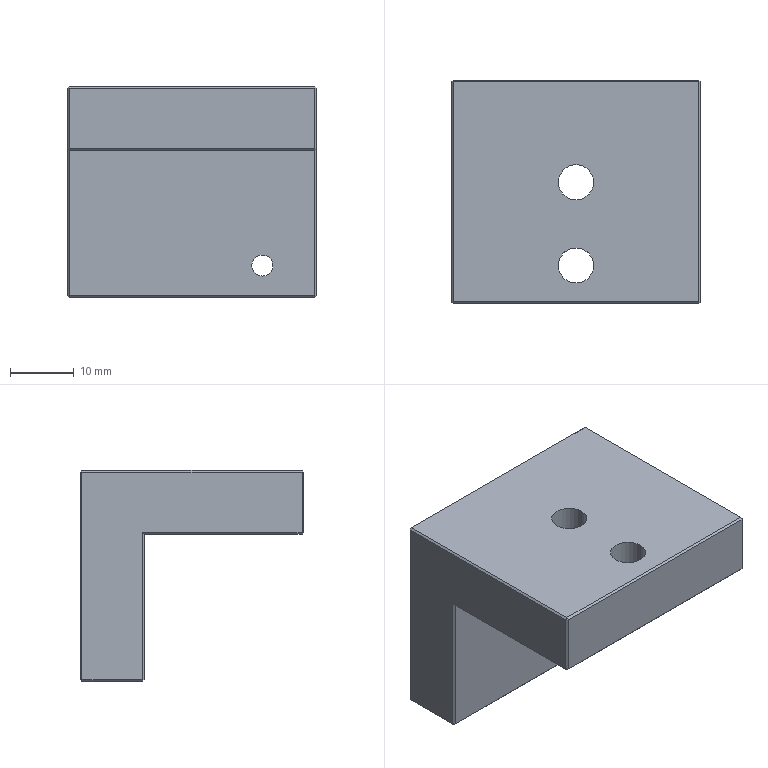Part | SolidWorks | features HoleWzd 2, Chamfer 1, Extrusion 1, ICE 1 | 1 solid | 51 faces | box 39 x 35 x 33 mm | volume 21329 mm3 | plane 37 | cylinder 12 | cone 2 | commonest cylinder face diameters 3.3 x4 5.5 x4 10 x4
STEP:
#1=CARTESIAN_POINT('',(5.,-6.,11.9));
#2=VERTEX_POINT('',#1);
#3=CARTESIAN_POINT('',(-5.,-6.,11.9));
#4=VERTEX_POINT('',#3);
#5=CARTESIAN_POINT('',(0.,-6.,11.9));
#6=DIRECTION('',(0.,0.,-1.));
#7=DIRECTION('',(-1.,0.,0.));
#8=AXIS2_PLACEMENT_3D('',#5,#6,#7);
#9=CIRCLE('',#8,5.);
#10=EDGE_CURVE('',#2,#4,#9,.T.);
#11=ORIENTED_EDGE('',*,*,#10,.F.);
#12=CARTESIAN_POINT('',(5.,-6.,6.5));
#13=VERTEX_POINT('',#12);
#14=CARTESIAN_POINT('',(5.,-6.,6.5));
#15=DIRECTION('',(0.,0.,-1.));
#16=VECTOR('',#15,1000.);
#17=LINE('',#14,#16);
#18=EDGE_CURVE('',#2,#13,#17,.T.);
#19=ORIENTED_EDGE('',*,*,#18,.T.);
#20=CARTESIAN_POINT('',(-5.,-6.,6.5));
#21=VERTEX_POINT('',#20);
#22=CARTESIAN_POINT('',(0.,-6.,6.5));
#23=DIRECTION('',(0.,0.,-1.));
#24=DIRECTION('',(-1.,0.,0.));
#25=AXIS2_PLACEMENT_3D('',#22,#23,#24);
#26=CIRCLE('',#25,5.);
#27=EDGE_CURVE('',#13,#21,#26,.T.);
#28=ORIENTED_EDGE('',*,*,#27,.T.);
#29=CARTESIAN_POINT('',(-5.,-6.,6.5));
#30=DIRECTION('',(0.,0.,-1.));
#31=VECTOR('',#30,1000.);
#32=LINE('',#29,#31);
#33=EDGE_CURVE('',#4,#21,#32,.T.);
#34=ORIENTED_EDGE('',*,*,#33,.F.);
#35=EDGE_LOOP('',(#11,#19,#28,#34));
#36=FACE_OUTER_BOUND('',#35,.T.);
#37=CARTESIAN_POINT('',(0.,-6.,6.5));
#38=DIRECTION('',(0.,0.,-1.));
#39=DIRECTION('',(-1.,0.,0.));
#40=AXIS2_PLACEMENT_3D('',#37,#38,#39);
#41=CYLINDRICAL_SURFACE('',#40,5.);
#42=ADVANCED_FACE('',(#36),#41,.F.);
#43=CARTESIAN_POINT('',(2.75,-6.,16.5));
#44=VERTEX_POINT('',#43);
#45=CARTESIAN_POINT('',(-2.75,-6.,16.5));
#46=VERTEX_POINT('',#45);
#47=CARTESIAN_POINT('',(0.,-6.,16.5));
#48=DIRECTION('',(0.,0.,-1.));
#49=DIRECTION('',(-1.,0.,0.));
#50=AXIS2_PLACEMENT_3D('',#47,#48,#49);
#51=CIRCLE('',#50,2.75);
#52=EDGE_CURVE('',#44,#46,#51,.T.);
#53=ORIENTED_EDGE('',*,*,#52,.F.);
#54=CARTESIAN_POINT('',(2.75,-6.,11.9));
#55=VERTEX_POINT('',#54);
#56=CARTESIAN_POINT('',(2.75,-6.,6.5));
#57=DIRECTION('',(0.,0.,-1.));
#58=VECTOR('',#57,1000.);
#59=LINE('',#56,#58);
#60=EDGE_CURVE('',#44,#55,#59,.T.);
#61=ORIENTED_EDGE('',*,*,#60,.T.);
#62=CARTESIAN_POINT('',(-2.75,-6.,11.9));
#63=VERTEX_POINT('',#62);
#64=CARTESIAN_POINT('',(0.,-6.,11.9));
#65=DIRECTION('',(0.,0.,-1.));
#66=DIRECTION('',(-1.,0.,0.));
#67=AXIS2_PLACEMENT_3D('',#64,#65,#66);
#68=CIRCLE('',#67,2.75);
#69=EDGE_CURVE('',#55,#63,#68,.T.);
#70=ORIENTED_EDGE('',*,*,#69,.T.);
#71=CARTESIAN_POINT('',(-2.75,-6.,6.5));
#72=DIRECTION('',(0.,0.,-1.));
#73=VECTOR('',#72,1000.);
#74=LINE('',#71,#73);
#75=EDGE_CURVE('',#46,#63,#74,.T.);
#76=ORIENTED_EDGE('',*,*,#75,.F.);
#77=EDGE_LOOP('',(#53,#61,#70,#76));
#78=FACE_OUTER_BOUND('',#77,.T.);
#79=CARTESIAN_POINT('',(0.,-6.,6.5));
#80=DIRECTION('',(0.,0.,-1.));
#81=DIRECTION('',(-1.,0.,0.));
#82=AXIS2_PLACEMENT_3D('',#79,#80,#81);
#83=CYLINDRICAL_SURFACE('',#82,2.75);
#84=ADVANCED_FACE('',(#78),#83,.F.);
#85=CARTESIAN_POINT('',(5.,-19.,11.9));
#86=VERTEX_POINT('',#85);
#87=CARTESIAN_POINT('',(-5.,-19.,11.9));
#88=VERTEX_POINT('',#87);
#89=CARTESIAN_POINT('',(0.,-19.,11.9));
#90=DIRECTION('',(0.,0.,-1.));
#91=DIRECTION('',(-1.,0.,0.));
#92=AXIS2_PLACEMENT_3D('',#89,#90,#91);
#93=CIRCLE('',#92,5.);
#94=EDGE_CURVE('',#86,#88,#93,.T.);
#95=ORIENTED_EDGE('',*,*,#94,.F.);
#96=CARTESIAN_POINT('',(5.,-19.,6.5));
#97=VERTEX_POINT('',#96);
#98=CARTESIAN_POINT('',(5.,-19.,6.5));
#99=DIRECTION('',(0.,0.,-1.));
#100=VECTOR('',#99,1000.);
#101=LINE('',#98,#100);
#102=EDGE_CURVE('',#86,#97,#101,.T.);
#103=ORIENTED_EDGE('',*,*,#102,.T.);
#104=CARTESIAN_POINT('',(-5.,-19.,6.5));
#105=VERTEX_POINT('',#104);
#106=CARTESIAN_POINT('',(0.,-19.,6.5));
#107=DIRECTION('',(0.,0.,-1.));
#108=DIRECTION('',(-1.,0.,0.));
#109=AXIS2_PLACEMENT_3D('',#106,#107,#108);
#110=CIRCLE('',#109,5.);
#111=EDGE_CURVE('',#97,#105,#110,.T.);
#112=ORIENTED_EDGE('',*,*,#111,.T.);
#113=CARTESIAN_POINT('',(-5.,-19.,6.5));
#114=DIRECTION('',(0.,0.,-1.));
#115=VECTOR('',#114,1000.);
#116=LINE('',#113,#115);
#117=EDGE_CURVE('',#88,#105,#116,.T.);
#118=ORIENTED_EDGE('',*,*,#117,.F.);
#119=EDGE_LOOP('',(#95,#103,#112,#118));
#120=FACE_OUTER_BOUND('',#119,.T.);
#121=CARTESIAN_POINT('',(0.,-19.,6.5));
#122=DIRECTION('',(0.,0.,-1.));
#123=DIRECTION('',(-1.,0.,0.));
#124=AXIS2_PLACEMENT_3D('',#121,#122,#123);
#125=CYLINDRICAL_SURFACE('',#124,5.);
#126=ADVANCED_FACE('',(#120),#125,.F.);
#127=CARTESIAN_POINT('',(2.75,-19.,16.5));
#128=VERTEX_POINT('',#127);
#129=CARTESIAN_POINT('',(-2.75,-19.,16.5));
#130=VERTEX_POINT('',#129);
#131=CARTESIAN_POINT('',(0.,-19.,16.5));
#132=DIRECTION('',(0.,0.,-1.));
#133=DIRECTION('',(-1.,0.,0.));
#134=AXIS2_PLACEMENT_3D('',#131,#132,#133);
#135=CIRCLE('',#134,2.75);
#136=EDGE_CURVE('',#128,#130,#135,.T.);
#137=ORIENTED_EDGE('',*,*,#136,.F.);
#138=CARTESIAN_POINT('',(2.75,-19.,11.9));
#139=VERTEX_POINT('',#138);
#140=CARTESIAN_POINT('',(2.75,-19.,6.5));
#141=DIRECTION('',(0.,0.,-1.));
#142=VECTOR('',#141,1000.);
#143=LINE('',#140,#142);
#144=EDGE_CURVE('',#128,#139,#143,.T.);
#145=ORIENTED_EDGE('',*,*,#144,.T.);
#146=CARTESIAN_POINT('',(-2.75,-19.,11.9));
#147=VERTEX_POINT('',#146);
#148=CARTESIAN_POINT('',(0.,-19.,11.9));
#149=DIRECTION('',(0.,0.,-1.));
#150=DIRECTION('',(-1.,0.,0.));
#151=AXIS2_PLACEMENT_3D('',#148,#149,#150);
#152=CIRCLE('',#151,2.75);
#153=EDGE_CURVE('',#139,#147,#152,.T.);
#154=ORIENTED_EDGE('',*,*,#153,.T.);
#155=CARTESIAN_POINT('',(-2.75,-19.,6.5));
#156=DIRECTION('',(0.,0.,-1.));
#157=VECTOR('',#156,1000.);
#158=LINE('',#155,#157);
#159=EDGE_CURVE('',#130,#147,#158,.T.);
#160=ORIENTED_EDGE('',*,*,#159,.F.);
#161=EDGE_LOOP('',(#137,#145,#154,#160));
#162=FACE_OUTER_BOUND('',#161,.T.);
#163=CARTESIAN_POINT('',(0.,-19.,6.5));
#164=DIRECTION('',(0.,0.,-1.));
#165=DIRECTION('',(-1.,0.,0.));
#166=AXIS2_PLACEMENT_3D('',#163,#164,#165);
#167=CYLINDRICAL_SURFACE('',#166,2.75);
#168=ADVANCED_FACE('',(#162),#167,.F.);
#169=CARTESIAN_POINT('',(11.,0.,-13.15));
#170=VERTEX_POINT('',#169);
#171=CARTESIAN_POINT('',(11.,0.,-9.85));
#172=VERTEX_POINT('',#171);
#173=CARTESIAN_POINT('',(11.,0.,-11.5));
#174=DIRECTION('',(0.,1.,0.));
#175=DIRECTION('',(0.,0.,1.));
#176=AXIS2_PLACEMENT_3D('',#173,#174,#175);
#177=CIRCLE('',#176,1.65);
#178=EDGE_CURVE('',#170,#172,#177,.T.);
#179=ORIENTED_EDGE('',*,*,#178,.F.);
#180=CARTESIAN_POINT('',(11.,10.,-13.15));
#181=VERTEX_POINT('',#180);
#182=CARTESIAN_POINT('',(11.,10.,-13.15));
#183=DIRECTION('',(0.,1.,0.));
#184=VECTOR('',#183,1000.);
#185=LINE('',#182,#184);
#186=EDGE_CURVE('',#170,#181,#185,.T.);
#187=ORIENTED_EDGE('',*,*,#186,.T.);
#188=CARTESIAN_POINT('',(11.,10.,-9.85));
#189=VERTEX_POINT('',#188);
#190=CARTESIAN_POINT('',(11.,10.,-11.5));
#191=DIRECTION('',(0.,1.,0.));
#192=DIRECTION('',(0.,0.,1.));
#193=AXIS2_PLACEMENT_3D('',#190,#191,#192);
#194=CIRCLE('',#193,1.65);
#195=EDGE_CURVE('',#181,#189,#194,.T.);
#196=ORIENTED_EDGE('',*,*,#195,.T.);
#197=CARTESIAN_POINT('',(11.,10.,-9.85));
#198=DIRECTION('',(0.,1.,0.));
#199=VECTOR('',#198,1000.);
#200=LINE('',#197,#199);
#201=EDGE_CURVE('',#172,#189,#200,.T.);
#202=ORIENTED_EDGE('',*,*,#201,.F.);
#203=EDGE_LOOP('',(#179,#187,#196,#202));
#204=FACE_OUTER_BOUND('',#203,.T.);
#205=CARTESIAN_POINT('',(11.,10.,-11.5));
#206=DIRECTION('',(0.,1.,0.));
#207=DIRECTION('',(0.,0.,1.));
#208=AXIS2_PLACEMENT_3D('',#205,#206,#207);
#209=CYLINDRICAL_SURFACE('',#208,1.65);
#210=ADVANCED_FACE('',(#204),#209,.F.);
#211=CARTESIAN_POINT('',(11.,-3.5,9.85));
#212=VERTEX_POINT('',#211);
#213=CARTESIAN_POINT('',(11.,-3.5,13.15));
#214=VERTEX_POINT('',#213);
#215=CARTESIAN_POINT('',(11.,-3.5,11.5));
#216=DIRECTION('',(0.,1.,0.));
#217=DIRECTION('',(0.,0.,1.));
#218=AXIS2_PLACEMENT_3D('',#215,#216,#217);
#219=CIRCLE('',#218,1.65);
#220=EDGE_CURVE('',#212,#214,#219,.T.);
#221=ORIENTED_EDGE('',*,*,#220,.F.);
#222=CARTESIAN_POINT('',(11.,10.,9.85));
#223=VERTEX_POINT('',#222);
#224=CARTESIAN_POINT('',(11.,10.,9.85));
#225=DIRECTION('',(0.,1.,0.));
#226=VECTOR('',#225,1000.);
#227=LINE('',#224,#226);
#228=EDGE_CURVE('',#212,#223,#227,.T.);
#229=ORIENTED_EDGE('',*,*,#228,.T.);
#230=CARTESIAN_POINT('',(11.,10.,13.15));
#231=VERTEX_POINT('',#230);
#232=CARTESIAN_POINT('',(11.,10.,11.5));
#233=DIRECTION('',(0.,1.,0.));
#234=DIRECTION('',(0.,0.,1.));
#235=AXIS2_PLACEMENT_3D('',#232,#233,#234);
#236=CIRCLE('',#235,1.65);
#237=EDGE_CURVE('',#223,#231,#236,.T.);
#238=ORIENTED_EDGE('',*,*,#237,.T.);
#239=CARTESIAN_POINT('',(11.,10.,13.15));
#240=DIRECTION('',(0.,1.,0.));
#241=VECTOR('',#240,1000.);
#242=LINE('',#239,#241);
#243=EDGE_CURVE('',#214,#231,#242,.T.);
#244=ORIENTED_EDGE('',*,*,#243,.F.);
#245=EDGE_LOOP('',(#221,#229,#238,#244));
#246=FACE_OUTER_BOUND('',#245,.T.);
#247=CARTESIAN_POINT('',(11.,10.,11.5));
#248=DIRECTION('',(0.,1.,0.));
#249=DIRECTION('',(0.,0.,1.));
#250=AXIS2_PLACEMENT_3D('',#247,#248,#249);
#251=CYLINDRICAL_SURFACE('',#250,1.65);
#252=ADVANCED_FACE('',(#246),#251,.F.);
#253=CARTESIAN_POINT('',(11.,-4.491,11.5));
#254=VERTEX_POINT('',#253);
#255=CARTESIAN_POINT('',(11.,-3.5,13.15));
#256=DIRECTION('',(0.,0.515,0.8572));
#257=VECTOR('',#256,1000.);
#258=LINE('',#255,#257);
#259=EDGE_CURVE('',#254,#214,#258,.T.);
#260=ORIENTED_EDGE('',*,*,#259,.F.);
#261=CARTESIAN_POINT('',(11.,-3.5,9.85));
#262=DIRECTION('',(0.,0.515,-0.8572));
#263=VECTOR('',#262,1000.);
#264=LINE('',#261,#263);
#265=EDGE_CURVE('',#254,#212,#264,.T.);
#266=ORIENTED_EDGE('',*,*,#265,.T.);
#267=ORIENTED_EDGE('',*,*,#220,.T.);
#268=EDGE_LOOP('',(#260,#266,#267));
#269=FACE_OUTER_BOUND('',#268,.T.);
#270=CARTESIAN_POINT('',(11.,-3.5,11.5));
#271=DIRECTION('',(0.,1.,0.));
#272=DIRECTION('',(0.,0.,1.));
#273=AXIS2_PLACEMENT_3D('',#270,#271,#272);
#274=CONICAL_SURFACE('',#273,1.65,1.03);
#275=ADVANCED_FACE('',(#269),#274,.F.);
#276=CARTESIAN_POINT('',(11.,0.,-11.5));
#277=DIRECTION('',(0.,1.,0.));
#278=DIRECTION('',(0.,0.,1.));
#279=AXIS2_PLACEMENT_3D('',#276,#277,#278);
#280=CIRCLE('',#279,1.65);
#281=EDGE_CURVE('',#172,#170,#280,.T.);
#282=ORIENTED_EDGE('',*,*,#281,.T.);
#283=ORIENTED_EDGE('',*,*,#178,.T.);
#284=EDGE_LOOP('',(#282,#283));
#285=FACE_BOUND('',#284,.T.);
#286=CARTESIAN_POINT('',(-19.2,0.,6.5));
#287=VERTEX_POINT('',#286);
#288=CARTESIAN_POINT('',(19.2,0.,6.5));
#289=VERTEX_POINT('',#288);
#290=CARTESIAN_POINT('',(-19.5,0.,6.5));
#291=DIRECTION('',(1.,0.,0.));
#292=VECTOR('',#291,1000.);
#293=LINE('',#290,#292);
#294=EDGE_CURVE('',#287,#289,#293,.T.);
#295=ORIENTED_EDGE('',*,*,#294,.F.);
#296=CARTESIAN_POINT('',(-19.2,0.,-16.2));
#297=VERTEX_POINT('',#296);
#298=CARTESIAN_POINT('',(-19.2,0.,0.));
#299=DIRECTION('',(0.,0.,-1.));
#300=VECTOR('',#299,1000.);
#301=LINE('',#298,#300);
#302=EDGE_CURVE('',#287,#297,#301,.T.);
#303=ORIENTED_EDGE('',*,*,#302,.T.);
#304=CARTESIAN_POINT('',(19.2,0.,-16.2));
#305=VERTEX_POINT('',#304);
#306=CARTESIAN_POINT('',(0.,0.,-16.2));
#307=DIRECTION('',(1.,0.,0.));
#308=VECTOR('',#307,1000.);
#309=LINE('',#306,#308);
#310=EDGE_CURVE('',#297,#305,#309,.T.);
#311=ORIENTED_EDGE('',*,*,#310,.T.);
#312=CARTESIAN_POINT('',(19.2,0.,0.));
#313=DIRECTION('',(0.,0.,1.));
#314=VECTOR('',#313,1000.);
#315=LINE('',#312,#314);
#316=EDGE_CURVE('',#305,#289,#315,.T.);
#317=ORIENTED_EDGE('',*,*,#316,.T.);
#318=EDGE_LOOP('',(#295,#303,#311,#317));
#319=FACE_OUTER_BOUND('',#318,.T.);
#320=CARTESIAN_POINT('',(0.,0.,0.));
#321=DIRECTION('',(0.,1.,0.));
#322=DIRECTION('',(0.,0.,1.));
#323=AXIS2_PLACEMENT_3D('',#320,#321,#322);
#324=PLANE('',#323);
#325=ADVANCED_FACE('',(#285,#319),#324,.F.);
#326=CARTESIAN_POINT('',(19.5,0.3,-16.2));
#327=VERTEX_POINT('',#326);
#328=CARTESIAN_POINT('',(19.5,9.7,-16.2));
#329=VERTEX_POINT('',#328);
#330=CARTESIAN_POINT('',(19.5,10.,-16.2));
#331=DIRECTION('',(0.,1.,0.));
#332=VECTOR('',#331,1000.);
#333=LINE('',#330,#332);
#334=EDGE_CURVE('',#327,#329,#333,.T.);
#335=ORIENTED_EDGE('',*,*,#334,.T.);
#336=CARTESIAN_POINT('',(19.5,9.7,16.2));
#337=VERTEX_POINT('',#336);
#338=CARTESIAN_POINT('',(19.5,9.7,16.5));
#339=DIRECTION('',(0.,0.,1.));
#340=VECTOR('',#339,1000.);
#341=LINE('',#338,#340);
#342=EDGE_CURVE('',#329,#337,#341,.T.);
#343=ORIENTED_EDGE('',*,*,#342,.T.);
#344=CARTESIAN_POINT('',(19.5,-24.7,16.2));
#345=VERTEX_POINT('',#344);
#346=CARTESIAN_POINT('',(19.5,10.,16.2));
#347=DIRECTION('',(0.,-1.,0.));
#348=VECTOR('',#347,1000.);
#349=LINE('',#346,#348);
#350=EDGE_CURVE('',#337,#345,#349,.T.);
#351=ORIENTED_EDGE('',*,*,#350,.T.);
#352=CARTESIAN_POINT('',(19.5,-24.7,6.8));
#353=VERTEX_POINT('',#352);
#354=CARTESIAN_POINT('',(19.5,-24.7,6.5));
#355=DIRECTION('',(0.,0.,-1.));
#356=VECTOR('',#355,1000.);
#357=LINE('',#354,#356);
#358=EDGE_CURVE('',#345,#353,#357,.T.);
#359=ORIENTED_EDGE('',*,*,#358,.T.);
#360=CARTESIAN_POINT('',(19.5,0.3,6.8));
#361=VERTEX_POINT('',#360);
#362=CARTESIAN_POINT('',(19.5,10.,6.8));
#363=DIRECTION('',(0.,1.,0.));
#364=VECTOR('',#363,1000.);
#365=LINE('',#362,#364);
#366=EDGE_CURVE('',#353,#361,#365,.T.);
#367=ORIENTED_EDGE('',*,*,#366,.T.);
#368=CARTESIAN_POINT('',(19.5,0.3,-16.5));
#369=DIRECTION('',(0.,0.,-1.));
#370=VECTOR('',#369,1000.);
#371=LINE('',#368,#370);
#372=EDGE_CURVE('',#361,#327,#371,.T.);
#373=ORIENTED_EDGE('',*,*,#372,.T.);
#374=EDGE_LOOP('',(#335,#343,#351,#359,#367,#373));
#375=FACE_OUTER_BOUND('',#374,.T.);
#376=CARTESIAN_POINT('',(19.5,10.,-16.5));
#377=DIRECTION('',(-1.,0.,0.));
#378=DIRECTION('',(0.,0.,1.));
#379=AXIS2_PLACEMENT_3D('',#376,#377,#378);
#380=PLANE('',#379);
#381=ADVANCED_FACE('',(#375),#380,.F.);
#382=CARTESIAN_POINT('',(19.2,0.3,-16.5));
#383=VERTEX_POINT('',#382);
#384=CARTESIAN_POINT('',(-19.2,0.3,-16.5));
#385=VERTEX_POINT('',#384);
#386=CARTESIAN_POINT('',(-19.5,0.3,-16.5));
#387=DIRECTION('',(-1.,0.,0.));
#388=VECTOR('',#387,1000.);
#389=LINE('',#386,#388);
#390=EDGE_CURVE('',#383,#385,#389,.T.);
#391=ORIENTED_EDGE('',*,*,#390,.T.);
#392=CARTESIAN_POINT('',(-19.2,9.7,-16.5));
#393=VERTEX_POINT('',#392);
#394=CARTESIAN_POINT('',(-19.2,10.,-16.5));
#395=DIRECTION('',(0.,1.,0.));
#396=VECTOR('',#395,1000.);
#397=LINE('',#394,#396);
#398=EDGE_CURVE('',#385,#393,#397,.T.);
#399=ORIENTED_EDGE('',*,*,#398,.T.);
#400=CARTESIAN_POINT('',(19.2,9.7,-16.5));
#401=VERTEX_POINT('',#400);
#402=CARTESIAN_POINT('',(19.5,9.7,-16.5));
#403=DIRECTION('',(1.,0.,0.));
#404=VECTOR('',#403,1000.);
#405=LINE('',#402,#404);
#406=EDGE_CURVE('',#393,#401,#405,.T.);
#407=ORIENTED_EDGE('',*,*,#406,.T.);
#408=CARTESIAN_POINT('',(19.2,10.,-16.5));
#409=DIRECTION('',(0.,-1.,0.));
#410=VECTOR('',#409,1000.);
#411=LINE('',#408,#410);
#412=EDGE_CURVE('',#401,#383,#411,.T.);
#413=ORIENTED_EDGE('',*,*,#412,.T.);
#414=EDGE_LOOP('',(#391,#399,#407,#413));
#415=FACE_OUTER_BOUND('',#414,.T.);
#416=CARTESIAN_POINT('',(-19.5,10.,-16.5));
#417=DIRECTION('',(0.,0.,1.));
#418=DIRECTION('',(1.,0.,0.));
#419=AXIS2_PLACEMENT_3D('',#416,#417,#418);
#420=PLANE('',#419);
#421=ADVANCED_FACE('',(#415),#420,.F.);
#422=CARTESIAN_POINT('',(-19.5,9.7,16.2));
#423=VERTEX_POINT('',#422);
#424=CARTESIAN_POINT('',(-19.5,9.7,-16.2));
#425=VERTEX_POINT('',#424);
#426=CARTESIAN_POINT('',(-19.5,9.7,-16.5));
#427=DIRECTION('',(0.,0.,-1.));
#428=VECTOR('',#427,1000.);
#429=LINE('',#426,#428);
#430=EDGE_CURVE('',#423,#425,#429,.T.);
#431=ORIENTED_EDGE('',*,*,#430,.T.);
#432=CARTESIAN_POINT('',(-19.5,0.3,-16.2));
#433=VERTEX_POINT('',#432);
#434=CARTESIAN_POINT('',(-19.5,10.,-16.2));
#435=DIRECTION('',(0.,-1.,0.));
#436=VECTOR('',#435,1000.);
#437=LINE('',#434,#436);
#438=EDGE_CURVE('',#425,#433,#437,.T.);
#439=ORIENTED_EDGE('',*,*,#438,.T.);
#440=CARTESIAN_POINT('',(-19.5,0.3,6.8));
#441=VERTEX_POINT('',#440);
#442=CARTESIAN_POINT('',(-19.5,0.3,-16.5));
#443=DIRECTION('',(0.,0.,1.));
#444=VECTOR('',#443,1000.);
#445=LINE('',#442,#444);
#446=EDGE_CURVE('',#433,#441,#445,.T.);
#447=ORIENTED_EDGE('',*,*,#446,.T.);
#448=CARTESIAN_POINT('',(-19.5,-24.7,6.8));
#449=VERTEX_POINT('',#448);
#450=CARTESIAN_POINT('',(-19.5,10.,6.8));
#451=DIRECTION('',(0.,-1.,0.));
#452=VECTOR('',#451,1000.);
#453=LINE('',#450,#452);
#454=EDGE_CURVE('',#441,#449,#453,.T.);
#455=ORIENTED_EDGE('',*,*,#454,.T.);
#456=CARTESIAN_POINT('',(-19.5,-24.7,16.2));
#457=VERTEX_POINT('',#456);
#458=CARTESIAN_POINT('',(-19.5,-24.7,16.5));
#459=DIRECTION('',(0.,0.,1.));
#460=VECTOR('',#459,1000.);
#461=LINE('',#458,#460);
#462=EDGE_CURVE('',#449,#457,#461,.T.);
#463=ORIENTED_EDGE('',*,*,#462,.T.);
#464=CARTESIAN_POINT('',(-19.5,10.,16.2));
#465=DIRECTION('',(0.,1.,0.));
#466=VECTOR('',#465,1000.);
#467=LINE('',#464,#466);
#468=EDGE_CURVE('',#457,#423,#467,.T.);
#469=ORIENTED_EDGE('',*,*,#468,.T.);
#470=EDGE_LOOP('',(#431,#439,#447,#455,#463,#469));
#471=FACE_OUTER_BOUND('',#470,.T.);
#472=CARTESIAN_POINT('',(-19.5,10.,-16.5));
#473=DIRECTION('',(1.,0.,0.));
#474=DIRECTION('',(0.,0.,-1.));
#475=AXIS2_PLACEMENT_3D('',#472,#473,#474);
#476=PLANE('',#475);
#477=ADVANCED_FACE('',(#471),#476,.F.);
#478=CARTESIAN_POINT('',(-19.2,9.7,16.5));
#479=VERTEX_POINT('',#478);
#480=CARTESIAN_POINT('',(-19.2,-24.7,16.5));
#481=VERTEX_POINT('',#480);
#482=CARTESIAN_POINT('',(-19.2,10.,16.5));
#483=DIRECTION('',(0.,-1.,0.));
#484=VECTOR('',#483,1000.);
#485=LINE('',#482,#484);
#486=EDGE_CURVE('',#479,#481,#485,.T.);
#487=ORIENTED_EDGE('',*,*,#486,.T.);
#488=CARTESIAN_POINT('',(19.2,-24.7,16.5));
#489=VERTEX_POINT('',#488);
#490=CARTESIAN_POINT('',(19.5,-24.7,16.5));
#491=DIRECTION('',(1.,0.,0.));
#492=VECTOR('',#491,1000.);
#493=LINE('',#490,#492);
#494=EDGE_CURVE('',#481,#489,#493,.T.);
#495=ORIENTED_EDGE('',*,*,#494,.T.);
#496=CARTESIAN_POINT('',(19.2,9.7,16.5));
#497=VERTEX_POINT('',#496);
#498=CARTESIAN_POINT('',(19.2,10.,16.5));
#499=DIRECTION('',(0.,1.,0.));
#500=VECTOR('',#499,1000.);
#501=LINE('',#498,#500);
#502=EDGE_CURVE('',#489,#497,#501,.T.);
#503=ORIENTED_EDGE('',*,*,#502,.T.);
#504=CARTESIAN_POINT('',(-19.5,9.7,16.5));
#505=DIRECTION('',(-1.,0.,0.));
#506=VECTOR('',#505,1000.);
#507=LINE('',#504,#506);
#508=EDGE_CURVE('',#497,#479,#507,.T.);
#509=ORIENTED_EDGE('',*,*,#508,.T.);
#510=EDGE_LOOP('',(#487,#495,#503,#509));
#511=FACE_OUTER_BOUND('',#510,.T.);
#512=CARTESIAN_POINT('',(0.,-6.,16.5));
#513=DIRECTION('',(0.,0.,-1.));
#514=DIRECTION('',(-1.,0.,0.));
#515=AXIS2_PLACEMENT_3D('',#512,#513,#514);
#516=CIRCLE('',#515,2.75);
#517=EDGE_CURVE('',#46,#44,#516,.T.);
#518=ORIENTED_EDGE('',*,*,#517,.T.);
#519=ORIENTED_EDGE('',*,*,#52,.T.);
#520=EDGE_LOOP('',(#518,#519));
#521=FACE_BOUND('',#520,.T.);
#522=CARTESIAN_POINT('',(0.,-19.,16.5));
#523=DIRECTION('',(0.,0.,-1.));
#524=DIRECTION('',(-1.,0.,0.));
#525=AXIS2_PLACEMENT_3D('',#522,#523,#524);
#526=CIRCLE('',#525,2.75);
#527=EDGE_CURVE('',#130,#128,#526,.T.);
#528=ORIENTED_EDGE('',*,*,#527,.T.);
#529=ORIENTED_EDGE('',*,*,#136,.T.);
#530=EDGE_LOOP('',(#528,#529));
#531=FACE_BOUND('',#530,.T.);
#532=CARTESIAN_POINT('',(-19.5,10.,16.5));
#533=DIRECTION('',(0.,0.,-1.));
#534=DIRECTION('',(-1.,0.,0.));
#535=AXIS2_PLACEMENT_3D('',#532,#533,#534);
#536=PLANE('',#535);
#537=ADVANCED_FACE('',(#511,#521,#531),#536,.F.);
#538=CARTESIAN_POINT('',(19.2,10.,16.2));
#539=VERTEX_POINT('',#538);
#540=CARTESIAN_POINT('',(19.2,10.,-16.2));
#541=VERTEX_POINT('',#540);
#542=CARTESIAN_POINT('',(19.2,10.,-16.5));
#543=DIRECTION('',(0.,0.,-1.));
#544=VECTOR('',#543,1000.);
#545=LINE('',#542,#544);
#546=EDGE_CURVE('',#539,#541,#545,.T.);
#547=ORIENTED_EDGE('',*,*,#546,.T.);
#548=CARTESIAN_POINT('',(-19.2,10.,-16.2));
#549=VERTEX_POINT('',#548);
#550=CARTESIAN_POINT('',(-19.5,10.,-16.2));
#551=DIRECTION('',(-1.,0.,0.));
#552=VECTOR('',#551,1000.);
#553=LINE('',#550,#552);
#554=EDGE_CURVE('',#541,#549,#553,.T.);
#555=ORIENTED_EDGE('',*,*,#554,.T.);
#556=CARTESIAN_POINT('',(-19.2,10.,16.2));
#557=VERTEX_POINT('',#556);
#558=CARTESIAN_POINT('',(-19.2,10.,16.5));
#559=DIRECTION('',(0.,0.,1.));
#560=VECTOR('',#559,1000.);
#561=LINE('',#558,#560);
#562=EDGE_CURVE('',#549,#557,#561,.T.);
#563=ORIENTED_EDGE('',*,*,#562,.T.);
#564=CARTESIAN_POINT('',(19.5,10.,16.2));
#565=DIRECTION('',(1.,0.,0.));
#566=VECTOR('',#565,1000.);
#567=LINE('',#564,#566);
#568=EDGE_CURVE('',#557,#539,#567,.T.);
#569=ORIENTED_EDGE('',*,*,#568,.T.);
#570=EDGE_LOOP('',(#547,#555,#563,#569));
#571=FACE_OUTER_BOUND('',#570,.T.);
#572=CARTESIAN_POINT('',(11.,10.,-11.5));
#573=DIRECTION('',(0.,1.,0.));
#574=DIRECTION('',(0.,0.,1.));
#575=AXIS2_PLACEMENT_3D('',#572,#573,#574);
#576=CIRCLE('',#575,1.65);
#577=EDGE_CURVE('',#189,#181,#576,.T.);
#578=ORIENTED_EDGE('',*,*,#577,.F.);
#579=ORIENTED_EDGE('',*,*,#195,.F.);
#580=EDGE_LOOP('',(#578,#579));
#581=FACE_BOUND('',#580,.T.);
#582=CARTESIAN_POINT('',(11.,10.,11.5));
#583=DIRECTION('',(0.,1.,0.));
#584=DIRECTION('',(0.,0.,1.));
#585=AXIS2_PLACEMENT_3D('',#582,#583,#584);
#586=CIRCLE('',#585,1.65);
#587=EDGE_CURVE('',#231,#223,#586,.T.);
#588=ORIENTED_EDGE('',*,*,#587,.F.);
#589=ORIENTED_EDGE('',*,*,#237,.F.);
#590=EDGE_LOOP('',(#588,#589));
#591=FACE_BOUND('',#590,.T.);
#592=CARTESIAN_POINT('',(0.,10.,0.));
#593=DIRECTION('',(0.,1.,0.));
#594=DIRECTION('',(0.,0.,1.));
#595=AXIS2_PLACEMENT_3D('',#592,#593,#594);
#596=PLANE('',#595);
#597=ADVANCED_FACE('',(#571,#581,#591),#596,.T.);
#598=CARTESIAN_POINT('',(0.,-6.,6.5));
#599=DIRECTION('',(0.,0.,-1.));
#600=DIRECTION('',(-1.,0.,0.));
#601=AXIS2_PLACEMENT_3D('',#598,#599,#600);
#602=CIRCLE('',#601,5.);
#603=EDGE_CURVE('',#21,#13,#602,.T.);
#604=ORIENTED_EDGE('',*,*,#603,.F.);
#605=ORIENTED_EDGE('',*,*,#27,.F.);
#606=EDGE_LOOP('',(#604,#605));
#607=FACE_BOUND('',#606,.T.);
#608=CARTESIAN_POINT('',(0.,-19.,6.5));
#609=DIRECTION('',(0.,0.,-1.));
#610=DIRECTION('',(-1.,0.,0.));
#611=AXIS2_PLACEMENT_3D('',#608,#609,#610);
#612=CIRCLE('',#611,5.);
#613=EDGE_CURVE('',#105,#97,#612,.T.);
#614=ORIENTED_EDGE('',*,*,#613,.F.);
#615=ORIENTED_EDGE('',*,*,#111,.F.);
#616=EDGE_LOOP('',(#614,#615));
#617=FACE_BOUND('',#616,.T.);
#618=CARTESIAN_POINT('',(19.2,-24.7,6.5));
#619=VERTEX_POINT('',#618);
#620=CARTESIAN_POINT('',(-19.2,-24.7,6.5));
#621=VERTEX_POINT('',#620);
#622=CARTESIAN_POINT('',(-19.5,-24.7,6.5));
#623=DIRECTION('',(-1.,0.,0.));
#624=VECTOR('',#623,1000.);
#625=LINE('',#622,#624);
#626=EDGE_CURVE('',#619,#621,#625,.T.);
#627=ORIENTED_EDGE('',*,*,#626,.T.);
#628=CARTESIAN_POINT('',(-19.2,-25.,6.5));
#629=DIRECTION('',(0.,1.,0.));
#630=VECTOR('',#629,1000.);
#631=LINE('',#628,#630);
#632=EDGE_CURVE('',#621,#287,#631,.T.);
#633=ORIENTED_EDGE('',*,*,#632,.T.);
#634=ORIENTED_EDGE('',*,*,#294,.T.);
#635=CARTESIAN_POINT('',(19.2,-25.,6.5));
#636=DIRECTION('',(0.,-1.,0.));
#637=VECTOR('',#636,1000.);
#638=LINE('',#635,#637);
#639=EDGE_CURVE('',#289,#619,#638,.T.);
#640=ORIENTED_EDGE('',*,*,#639,.T.);
#641=EDGE_LOOP('',(#627,#633,#634,#640));
#642=FACE_OUTER_BOUND('',#641,.T.);
#643=CARTESIAN_POINT('',(-19.5,-25.,6.5));
#644=DIRECTION('',(0.,0.,1.));
#645=DIRECTION('',(1.,0.,0.));
#646=AXIS2_PLACEMENT_3D('',#643,#644,#645);
#647=PLANE('',#646);
#648=ADVANCED_FACE('',(#607,#617,#642),#647,.F.);
#649=CARTESIAN_POINT('',(19.2,-25.,16.2));
#650=VERTEX_POINT('',#649);
#651=CARTESIAN_POINT('',(-19.2,-25.,16.2));
#652=VERTEX_POINT('',#651);
#653=CARTESIAN_POINT('',(-19.5,-25.,16.2));
#654=DIRECTION('',(-1.,0.,0.));
#655=VECTOR('',#654,1000.);
#656=LINE('',#653,#655);
#657=EDGE_CURVE('',#650,#652,#656,.T.);
#658=ORIENTED_EDGE('',*,*,#657,.T.);
#659=CARTESIAN_POINT('',(-19.2,-25.,6.8));
#660=VERTEX_POINT('',#659);
#661=CARTESIAN_POINT('',(-19.2,-25.,6.5));
#662=DIRECTION('',(0.,0.,-1.));
#663=VECTOR('',#662,1000.);
#664=LINE('',#661,#663);
#665=EDGE_CURVE('',#652,#660,#664,.T.);
#666=ORIENTED_EDGE('',*,*,#665,.T.);
#667=CARTESIAN_POINT('',(19.2,-25.,6.8));
#668=VERTEX_POINT('',#667);
#669=CARTESIAN_POINT('',(19.5,-25.,6.8));
#670=DIRECTION('',(1.,0.,0.));
#671=VECTOR('',#670,1000.);
#672=LINE('',#669,#671);
#673=EDGE_CURVE('',#660,#668,#672,.T.);
#674=ORIENTED_EDGE('',*,*,#673,.T.);
#675=CARTESIAN_POINT('',(19.2,-25.,16.5));
#676=DIRECTION('',(0.,0.,1.));
#677=VECTOR('',#676,1000.);
#678=LINE('',#675,#677);
#679=EDGE_CURVE('',#668,#650,#678,.T.);
#680=ORIENTED_EDGE('',*,*,#679,.T.);
#681=EDGE_LOOP('',(#658,#666,#674,#680));
#682=FACE_OUTER_BOUND('',#681,.T.);
#683=CARTESIAN_POINT('',(0.,-25.,0.));
#684=DIRECTION('',(0.,-1.,0.));
#685=DIRECTION('',(0.,0.,-1.));
#686=AXIS2_PLACEMENT_3D('',#683,#684,#685);
#687=PLANE('',#686);
#688=ADVANCED_FACE('',(#682),#687,.T.);
#689=ORIENTED_EDGE('',*,*,#265,.F.);
#690=ORIENTED_EDGE('',*,*,#259,.T.);
#691=CARTESIAN_POINT('',(11.,-3.5,11.5));
#692=DIRECTION('',(0.,1.,0.));
#693=DIRECTION('',(0.,0.,1.));
#694=AXIS2_PLACEMENT_3D('',#691,#692,#693);
#695=CIRCLE('',#694,1.65);
#696=EDGE_CURVE('',#214,#212,#695,.T.);
#697=ORIENTED_EDGE('',*,*,#696,.T.);
#698=EDGE_LOOP('',(#689,#690,#697));
#699=FACE_OUTER_BOUND('',#698,.T.);
#700=CARTESIAN_POINT('',(11.,-3.5,11.5));
#701=DIRECTION('',(0.,1.,0.));
#702=DIRECTION('',(0.,0.,1.));
#703=AXIS2_PLACEMENT_3D('',#700,#701,#702);
#704=CONICAL_SURFACE('',#703,1.65,1.03);
#705=ADVANCED_FACE('',(#699),#704,.F.);
#706=ORIENTED_EDGE('',*,*,#228,.F.);
#707=ORIENTED_EDGE('',*,*,#696,.F.);
#708=ORIENTED_EDGE('',*,*,#243,.T.);
#709=ORIENTED_EDGE('',*,*,#587,.T.);
#710=EDGE_LOOP('',(#706,#707,#708,#709));
#711=FACE_OUTER_BOUND('',#710,.T.);
#712=CARTESIAN_POINT('',(11.,10.,11.5));
#713=DIRECTION('',(0.,1.,0.));
#714=DIRECTION('',(0.,0.,1.));
#715=AXIS2_PLACEMENT_3D('',#712,#713,#714);
#716=CYLINDRICAL_SURFACE('',#715,1.65);
#717=ADVANCED_FACE('',(#711),#716,.F.);
#718=ORIENTED_EDGE('',*,*,#186,.F.);
#719=ORIENTED_EDGE('',*,*,#281,.F.);
#720=ORIENTED_EDGE('',*,*,#201,.T.);
#721=ORIENTED_EDGE('',*,*,#577,.T.);
#722=EDGE_LOOP('',(#718,#719,#720,#721));
#723=FACE_OUTER_BOUND('',#722,.T.);
#724=CARTESIAN_POINT('',(11.,10.,-11.5));
#725=DIRECTION('',(0.,1.,0.));
#726=DIRECTION('',(0.,0.,1.));
#727=AXIS2_PLACEMENT_3D('',#724,#725,#726);
#728=CYLINDRICAL_SURFACE('',#727,1.65);
#729=ADVANCED_FACE('',(#723),#728,.F.);
#730=ORIENTED_EDGE('',*,*,#144,.F.);
#731=ORIENTED_EDGE('',*,*,#527,.F.);
#732=ORIENTED_EDGE('',*,*,#159,.T.);
#733=CARTESIAN_POINT('',(0.,-19.,11.9));
#734=DIRECTION('',(0.,0.,-1.));
#735=DIRECTION('',(-1.,0.,0.));
#736=AXIS2_PLACEMENT_3D('',#733,#734,#735);
#737=CIRCLE('',#736,2.75);
#738=EDGE_CURVE('',#147,#139,#737,.T.);
#739=ORIENTED_EDGE('',*,*,#738,.T.);
#740=EDGE_LOOP('',(#730,#731,#732,#739));
#741=FACE_OUTER_BOUND('',#740,.T.);
#742=CARTESIAN_POINT('',(0.,-19.,6.5));
#743=DIRECTION('',(0.,0.,-1.));
#744=DIRECTION('',(-1.,0.,0.));
#745=AXIS2_PLACEMENT_3D('',#742,#743,#744);
#746=CYLINDRICAL_SURFACE('',#745,2.75);
#747=ADVANCED_FACE('',(#741),#746,.F.);
#748=ORIENTED_EDGE('',*,*,#738,.F.);
#749=ORIENTED_EDGE('',*,*,#153,.F.);
#750=EDGE_LOOP('',(#748,#749));
#751=FACE_BOUND('',#750,.T.);
#752=CARTESIAN_POINT('',(0.,-19.,11.9));
#753=DIRECTION('',(0.,0.,-1.));
#754=DIRECTION('',(-1.,0.,0.));
#755=AXIS2_PLACEMENT_3D('',#752,#753,#754);
#756=CIRCLE('',#755,5.);
#757=EDGE_CURVE('',#88,#86,#756,.T.);
#758=ORIENTED_EDGE('',*,*,#757,.T.);
#759=ORIENTED_EDGE('',*,*,#94,.T.);
#760=EDGE_LOOP('',(#758,#759));
#761=FACE_OUTER_BOUND('',#760,.T.);
#762=CARTESIAN_POINT('',(2.75,-19.,11.9));
#763=DIRECTION('',(0.,0.,1.));
#764=DIRECTION('',(1.,0.,0.));
#765=AXIS2_PLACEMENT_3D('',#762,#763,#764);
#766=PLANE('',#765);
#767=ADVANCED_FACE('',(#751,#761),#766,.F.);
#768=ORIENTED_EDGE('',*,*,#102,.F.);
#769=ORIENTED_EDGE('',*,*,#757,.F.);
#770=ORIENTED_EDGE('',*,*,#117,.T.);
#771=ORIENTED_EDGE('',*,*,#613,.T.);
#772=EDGE_LOOP('',(#768,#769,#770,#771));
#773=FACE_OUTER_BOUND('',#772,.T.);
#774=CARTESIAN_POINT('',(0.,-19.,6.5));
#775=DIRECTION('',(0.,0.,-1.));
#776=DIRECTION('',(-1.,0.,0.));
#777=AXIS2_PLACEMENT_3D('',#774,#775,#776);
#778=CYLINDRICAL_SURFACE('',#777,5.);
#779=ADVANCED_FACE('',(#773),#778,.F.);
#780=ORIENTED_EDGE('',*,*,#60,.F.);
#781=ORIENTED_EDGE('',*,*,#517,.F.);
#782=ORIENTED_EDGE('',*,*,#75,.T.);
#783=CARTESIAN_POINT('',(0.,-6.,11.9));
#784=DIRECTION('',(0.,0.,-1.));
#785=DIRECTION('',(-1.,0.,0.));
#786=AXIS2_PLACEMENT_3D('',#783,#784,#785);
#787=CIRCLE('',#786,2.75);
#788=EDGE_CURVE('',#63,#55,#787,.T.);
#789=ORIENTED_EDGE('',*,*,#788,.T.);
#790=EDGE_LOOP('',(#780,#781,#782,#789));
#791=FACE_OUTER_BOUND('',#790,.T.);
#792=CARTESIAN_POINT('',(0.,-6.,6.5));
#793=DIRECTION('',(0.,0.,-1.));
#794=DIRECTION('',(-1.,0.,0.));
#795=AXIS2_PLACEMENT_3D('',#792,#793,#794);
#796=CYLINDRICAL_SURFACE('',#795,2.75);
#797=ADVANCED_FACE('',(#791),#796,.F.);
#798=ORIENTED_EDGE('',*,*,#788,.F.);
#799=ORIENTED_EDGE('',*,*,#69,.F.);
#800=EDGE_LOOP('',(#798,#799));
#801=FACE_BOUND('',#800,.T.);
#802=CARTESIAN_POINT('',(0.,-6.,11.9));
#803=DIRECTION('',(0.,0.,-1.));
#804=DIRECTION('',(-1.,0.,0.));
#805=AXIS2_PLACEMENT_3D('',#802,#803,#804);
#806=CIRCLE('',#805,5.);
#807=EDGE_CURVE('',#4,#2,#806,.T.);
#808=ORIENTED_EDGE('',*,*,#807,.T.);
#809=ORIENTED_EDGE('',*,*,#10,.T.);
#810=EDGE_LOOP('',(#808,#809));
#811=FACE_OUTER_BOUND('',#810,.T.);
#812=CARTESIAN_POINT('',(2.75,-6.,11.9));
#813=DIRECTION('',(0.,0.,1.));
#814=DIRECTION('',(1.,0.,0.));
#815=AXIS2_PLACEMENT_3D('',#812,#813,#814);
#816=PLANE('',#815);
#817=ADVANCED_FACE('',(#801,#811),#816,.F.);
#818=ORIENTED_EDGE('',*,*,#18,.F.);
#819=ORIENTED_EDGE('',*,*,#807,.F.);
#820=ORIENTED_EDGE('',*,*,#33,.T.);
#821=ORIENTED_EDGE('',*,*,#603,.T.);
#822=EDGE_LOOP('',(#818,#819,#820,#821));
#823=FACE_OUTER_BOUND('',#822,.T.);
#824=CARTESIAN_POINT('',(0.,-6.,6.5));
#825=DIRECTION('',(0.,0.,-1.));
#826=DIRECTION('',(-1.,0.,0.));
#827=AXIS2_PLACEMENT_3D('',#824,#825,#826);
#828=CYLINDRICAL_SURFACE('',#827,5.);
#829=ADVANCED_FACE('',(#823),#828,.F.);
#830=CARTESIAN_POINT('',(-19.2,0.3,-16.5));
#831=DIRECTION('',(0.,-0.7071,0.7071));
#832=VECTOR('',#831,1000.);
#833=LINE('',#830,#832);
#834=EDGE_CURVE('',#385,#297,#833,.T.);
#835=ORIENTED_EDGE('',*,*,#834,.F.);
#836=ORIENTED_EDGE('',*,*,#390,.F.);
#837=CARTESIAN_POINT('',(19.2,0.,-16.2));
#838=DIRECTION('',(0.,0.7071,-0.7071));
#839=VECTOR('',#838,1000.);
#840=LINE('',#837,#839);
#841=EDGE_CURVE('',#305,#383,#840,.T.);
#842=ORIENTED_EDGE('',*,*,#841,.F.);
#843=ORIENTED_EDGE('',*,*,#310,.F.);
#844=EDGE_LOOP('',(#835,#836,#842,#843));
#845=FACE_OUTER_BOUND('',#844,.T.);
#846=CARTESIAN_POINT('',(-19.5,0.3,-16.5));
#847=DIRECTION('',(0.,0.7071,0.7071));
#848=DIRECTION('',(-1.,0.,0.));
#849=AXIS2_PLACEMENT_3D('',#846,#847,#848);
#850=PLANE('',#849);
#851=ADVANCED_FACE('',(#845),#850,.F.);
#852=CARTESIAN_POINT('',(19.35,0.3,-16.35));
#853=DIRECTION('',(0.7071,0.,0.7071));
#854=VECTOR('',#853,1000.);
#855=LINE('',#852,#854);
#856=EDGE_CURVE('',#383,#327,#855,.T.);
#857=ORIENTED_EDGE('',*,*,#856,.F.);
#858=ORIENTED_EDGE('',*,*,#412,.F.);
#859=CARTESIAN_POINT('',(19.2,9.7,-16.5));
#860=DIRECTION('',(-0.7071,0.,-0.7071));
#861=VECTOR('',#860,1000.);
#862=LINE('',#859,#861);
#863=EDGE_CURVE('',#329,#401,#862,.T.);
#864=ORIENTED_EDGE('',*,*,#863,.F.);
#865=ORIENTED_EDGE('',*,*,#334,.F.);
#866=EDGE_LOOP('',(#857,#858,#864,#865));
#867=FACE_OUTER_BOUND('',#866,.T.);
#868=CARTESIAN_POINT('',(19.2,10.,-16.5));
#869=DIRECTION('',(-0.7071,0.,0.7071));
#870=DIRECTION('',(0.,-1.,0.));
#871=AXIS2_PLACEMENT_3D('',#868,#869,#870);
#872=PLANE('',#871);
#873=ADVANCED_FACE('',(#867),#872,.F.);
#874=ORIENTED_EDGE('',*,*,#841,.T.);
#875=ORIENTED_EDGE('',*,*,#856,.T.);
#876=CARTESIAN_POINT('',(19.2,0.,-16.2));
#877=DIRECTION('',(0.7071,0.7071,0.));
#878=VECTOR('',#877,1000.);
#879=LINE('',#876,#878);
#880=EDGE_CURVE('',#305,#327,#879,.T.);
#881=ORIENTED_EDGE('',*,*,#880,.F.);
#882=EDGE_LOOP('',(#874,#875,#881));
#883=FACE_OUTER_BOUND('',#882,.T.);
#884=CARTESIAN_POINT('',(19.2,0.,-16.2));
#885=DIRECTION('',(0.5774,-0.5774,-0.5774));
#886=DIRECTION('',(-0.7071,0.,-0.7071));
#887=AXIS2_PLACEMENT_3D('',#884,#885,#886);
#888=PLANE('',#887);
#889=ADVANCED_FACE('',(#883),#888,.T.);
#890=CARTESIAN_POINT('',(-19.35,0.15,-16.2));
#891=DIRECTION('',(0.7071,-0.7071,0.));
#892=VECTOR('',#891,1000.);
#893=LINE('',#890,#892);
#894=EDGE_CURVE('',#433,#297,#893,.T.);
#895=ORIENTED_EDGE('',*,*,#894,.F.);
#896=CARTESIAN_POINT('',(-19.2,0.3,-16.5));
#897=DIRECTION('',(-0.7071,0.,0.7071));
#898=VECTOR('',#897,1000.);
#899=LINE('',#896,#898);
#900=EDGE_CURVE('',#385,#433,#899,.T.);
#901=ORIENTED_EDGE('',*,*,#900,.F.);
#902=ORIENTED_EDGE('',*,*,#834,.T.);
#903=EDGE_LOOP('',(#895,#901,#902));
#904=FACE_OUTER_BOUND('',#903,.T.);
#905=CARTESIAN_POINT('',(-19.2,0.3,-16.5));
#906=DIRECTION('',(-0.5774,-0.5774,-0.5774));
#907=DIRECTION('',(0.,0.7071,-0.7071));
#908=AXIS2_PLACEMENT_3D('',#905,#906,#907);
#909=PLANE('',#908);
#910=ADVANCED_FACE('',(#904),#909,.T.);
#911=ORIENTED_EDGE('',*,*,#900,.T.);
#912=ORIENTED_EDGE('',*,*,#438,.F.);
#913=CARTESIAN_POINT('',(-19.35,9.7,-16.35));
#914=DIRECTION('',(-0.7071,0.,0.7071));
#915=VECTOR('',#914,1000.);
#916=LINE('',#913,#915);
#917=EDGE_CURVE('',#393,#425,#916,.T.);
#918=ORIENTED_EDGE('',*,*,#917,.F.);
#919=ORIENTED_EDGE('',*,*,#398,.F.);
#920=EDGE_LOOP('',(#911,#912,#918,#919));
#921=FACE_OUTER_BOUND('',#920,.T.);
#922=CARTESIAN_POINT('',(-19.5,10.,-16.2));
#923=DIRECTION('',(0.7071,0.,0.7071));
#924=DIRECTION('',(0.,-1.,0.));
#925=AXIS2_PLACEMENT_3D('',#922,#923,#924);
#926=PLANE('',#925);
#927=ADVANCED_FACE('',(#921),#926,.F.);
#928=CARTESIAN_POINT('',(19.2,9.7,-16.5));
#929=DIRECTION('',(0.,0.7071,0.7071));
#930=VECTOR('',#929,1000.);
#931=LINE('',#928,#930);
#932=EDGE_CURVE('',#401,#541,#931,.T.);
#933=ORIENTED_EDGE('',*,*,#932,.F.);
#934=ORIENTED_EDGE('',*,*,#406,.F.);
#935=CARTESIAN_POINT('',(-19.2,10.,-16.2));
#936=DIRECTION('',(0.,-0.7071,-0.7071));
#937=VECTOR('',#936,1000.);
#938=LINE('',#935,#937);
#939=EDGE_CURVE('',#549,#393,#938,.T.);
#940=ORIENTED_EDGE('',*,*,#939,.F.);
#941=ORIENTED_EDGE('',*,*,#554,.F.);
#942=EDGE_LOOP('',(#933,#934,#940,#941));
#943=FACE_OUTER_BOUND('',#942,.T.);
#944=CARTESIAN_POINT('',(0.,10.,-16.2));
#945=DIRECTION('',(0.,0.7071,-0.7071));
#946=DIRECTION('',(1.,0.,0.));
#947=AXIS2_PLACEMENT_3D('',#944,#945,#946);
#948=PLANE('',#947);
#949=ADVANCED_FACE('',(#943),#948,.T.);
#950=ORIENTED_EDGE('',*,*,#863,.T.);
#951=ORIENTED_EDGE('',*,*,#932,.T.);
#952=CARTESIAN_POINT('',(19.35,9.85,-16.2));
#953=DIRECTION('',(-0.7071,0.7071,0.));
#954=VECTOR('',#953,1000.);
#955=LINE('',#952,#954);
#956=EDGE_CURVE('',#329,#541,#955,.T.);
#957=ORIENTED_EDGE('',*,*,#956,.F.);
#958=EDGE_LOOP('',(#950,#951,#957));
#959=FACE_OUTER_BOUND('',#958,.T.);
#960=CARTESIAN_POINT('',(19.2,9.7,-16.5));
#961=DIRECTION('',(0.5774,0.5774,-0.5774));
#962=DIRECTION('',(-0.7071,0.,-0.7071));
#963=AXIS2_PLACEMENT_3D('',#960,#961,#962);
#964=PLANE('',#963);
#965=ADVANCED_FACE('',(#959),#964,.T.);
#966=ORIENTED_EDGE('',*,*,#880,.T.);
#967=ORIENTED_EDGE('',*,*,#372,.F.);
#968=CARTESIAN_POINT('',(11.733,-7.467,-0.9667));
#969=DIRECTION('',(0.5774,0.5774,0.5774));
#970=VECTOR('',#969,1000.);
#971=LINE('',#968,#970);
#972=EDGE_CURVE('',#289,#361,#971,.T.);
#973=ORIENTED_EDGE('',*,*,#972,.F.);
#974=ORIENTED_EDGE('',*,*,#316,.F.);
#975=EDGE_LOOP('',(#966,#967,#973,#974));
#976=FACE_OUTER_BOUND('',#975,.T.);
#977=CARTESIAN_POINT('',(19.5,0.3,-16.5));
#978=DIRECTION('',(-0.7071,0.7071,0.));
#979=DIRECTION('',(0.,0.,-1.));
#980=AXIS2_PLACEMENT_3D('',#977,#978,#979);
#981=PLANE('',#980);
#982=ADVANCED_FACE('',(#976),#981,.F.);
#983=ORIENTED_EDGE('',*,*,#894,.T.);
#984=ORIENTED_EDGE('',*,*,#302,.F.);
#985=CARTESIAN_POINT('',(-11.733,-7.467,-0.9667));
#986=DIRECTION('',(0.5774,-0.5774,-0.5774));
#987=VECTOR('',#986,1000.);
#988=LINE('',#985,#987);
#989=EDGE_CURVE('',#441,#287,#988,.T.);
#990=ORIENTED_EDGE('',*,*,#989,.F.);
#991=ORIENTED_EDGE('',*,*,#446,.F.);
#992=EDGE_LOOP('',(#983,#984,#990,#991));
#993=FACE_OUTER_BOUND('',#992,.T.);
#994=CARTESIAN_POINT('',(-19.5,0.3,-16.5));
#995=DIRECTION('',(0.7071,0.7071,0.));
#996=DIRECTION('',(0.,0.,1.));
#997=AXIS2_PLACEMENT_3D('',#994,#995,#996);
#998=PLANE('',#997);
#999=ADVANCED_FACE('',(#993),#998,.F.);
#1000=ORIENTED_EDGE('',*,*,#939,.T.);
#1001=ORIENTED_EDGE('',*,*,#917,.T.);
#1002=CARTESIAN_POINT('',(-19.2,10.,-16.2));
#1003=DIRECTION('',(-0.7071,-0.7071,0.));
#1004=VECTOR('',#1003,1000.);
#1005=LINE('',#1002,#1004);
#1006=EDGE_CURVE('',#549,#425,#1005,.T.);
#1007=ORIENTED_EDGE('',*,*,#1006,.F.);
#1008=EDGE_LOOP('',(#1000,#1001,#1007));
#1009=FACE_OUTER_BOUND('',#1008,.T.);
#1010=CARTESIAN_POINT('',(-19.2,10.,-16.2));
#1011=DIRECTION('',(-0.5774,0.5774,-0.5774));
#1012=DIRECTION('',(-0.7071,0.,0.7071));
#1013=AXIS2_PLACEMENT_3D('',#1010,#1011,#1012);
#1014=PLANE('',#1013);
#1015=ADVANCED_FACE('',(#1009),#1014,.T.);
#1016=ORIENTED_EDGE('',*,*,#956,.T.);
#1017=ORIENTED_EDGE('',*,*,#546,.F.);
#1018=CARTESIAN_POINT('',(19.5,9.7,16.2));
#1019=DIRECTION('',(-0.7071,0.7071,0.));
#1020=VECTOR('',#1019,1000.);
#1021=LINE('',#1018,#1020);
#1022=EDGE_CURVE('',#337,#539,#1021,.T.);
#1023=ORIENTED_EDGE('',*,*,#1022,.F.);
#1024=ORIENTED_EDGE('',*,*,#342,.F.);
#1025=EDGE_LOOP('',(#1016,#1017,#1023,#1024));
#1026=FACE_OUTER_BOUND('',#1025,.T.);
#1027=CARTESIAN_POINT('',(19.2,10.,0.));
#1028=DIRECTION('',(0.7071,0.7071,0.));
#1029=DIRECTION('',(0.,0.,1.));
#1030=AXIS2_PLACEMENT_3D('',#1027,#1028,#1029);
#1031=PLANE('',#1030);
#1032=ADVANCED_FACE('',(#1026),#1031,.T.);
#1033=ORIENTED_EDGE('',*,*,#972,.T.);
#1034=ORIENTED_EDGE('',*,*,#366,.F.);
#1035=CARTESIAN_POINT('',(19.35,-24.7,6.65));
#1036=DIRECTION('',(0.7071,0.,0.7071));
#1037=VECTOR('',#1036,1000.);
#1038=LINE('',#1035,#1037);
#1039=EDGE_CURVE('',#619,#353,#1038,.T.);
#1040=ORIENTED_EDGE('',*,*,#1039,.F.);
#1041=ORIENTED_EDGE('',*,*,#639,.F.);
#1042=EDGE_LOOP('',(#1033,#1034,#1040,#1041));
#1043=FACE_OUTER_BOUND('',#1042,.T.);
#1044=CARTESIAN_POINT('',(19.5,10.,6.8));
#1045=DIRECTION('',(-0.7071,0.,0.7071));
#1046=DIRECTION('',(0.,1.,0.));
#1047=AXIS2_PLACEMENT_3D('',#1044,#1045,#1046);
#1048=PLANE('',#1047);
#1049=ADVANCED_FACE('',(#1043),#1048,.F.);
#1050=CARTESIAN_POINT('',(-19.2,-24.7,6.5));
#1051=DIRECTION('',(0.,-0.7071,0.7071));
#1052=VECTOR('',#1051,1000.);
#1053=LINE('',#1050,#1052);
#1054=EDGE_CURVE('',#621,#660,#1053,.T.);
#1055=ORIENTED_EDGE('',*,*,#1054,.F.);
#1056=ORIENTED_EDGE('',*,*,#626,.F.);
#1057=CARTESIAN_POINT('',(19.2,-25.,6.8));
#1058=DIRECTION('',(0.,0.7071,-0.7071));
#1059=VECTOR('',#1058,1000.);
#1060=LINE('',#1057,#1059);
#1061=EDGE_CURVE('',#668,#619,#1060,.T.);
#1062=ORIENTED_EDGE('',*,*,#1061,.F.);
#1063=ORIENTED_EDGE('',*,*,#673,.F.);
#1064=EDGE_LOOP('',(#1055,#1056,#1062,#1063));
#1065=FACE_OUTER_BOUND('',#1064,.T.);
#1066=CARTESIAN_POINT('',(0.,-25.,6.8));
#1067=DIRECTION('',(0.,-0.7071,-0.7071));
#1068=DIRECTION('',(-1.,0.,0.));
#1069=AXIS2_PLACEMENT_3D('',#1066,#1067,#1068);
#1070=PLANE('',#1069);
#1071=ADVANCED_FACE('',(#1065),#1070,.T.);
#1072=ORIENTED_EDGE('',*,*,#989,.T.);
#1073=ORIENTED_EDGE('',*,*,#632,.F.);
#1074=CARTESIAN_POINT('',(-19.2,-24.7,6.5));
#1075=DIRECTION('',(0.7071,0.,-0.7071));
#1076=VECTOR('',#1075,1000.);
#1077=LINE('',#1074,#1076);
#1078=EDGE_CURVE('',#449,#621,#1077,.T.);
#1079=ORIENTED_EDGE('',*,*,#1078,.F.);
#1080=ORIENTED_EDGE('',*,*,#454,.F.);
#1081=EDGE_LOOP('',(#1072,#1073,#1079,#1080));
#1082=FACE_OUTER_BOUND('',#1081,.T.);
#1083=CARTESIAN_POINT('',(-19.2,-25.,6.5));
#1084=DIRECTION('',(0.7071,0.,0.7071));
#1085=DIRECTION('',(0.,1.,0.));
#1086=AXIS2_PLACEMENT_3D('',#1083,#1084,#1085);
#1087=PLANE('',#1086);
#1088=ADVANCED_FACE('',(#1082),#1087,.F.);
#1089=ORIENTED_EDGE('',*,*,#1006,.T.);
#1090=ORIENTED_EDGE('',*,*,#430,.F.);
#1091=CARTESIAN_POINT('',(-19.2,10.,16.2));
#1092=DIRECTION('',(-0.7071,-0.7071,0.));
#1093=VECTOR('',#1092,1000.);
#1094=LINE('',#1091,#1093);
#1095=EDGE_CURVE('',#557,#423,#1094,.T.);
#1096=ORIENTED_EDGE('',*,*,#1095,.F.);
#1097=ORIENTED_EDGE('',*,*,#562,.F.);
#1098=EDGE_LOOP('',(#1089,#1090,#1096,#1097));
#1099=FACE_OUTER_BOUND('',#1098,.T.);
#1100=CARTESIAN_POINT('',(-19.2,10.,0.));
#1101=DIRECTION('',(-0.7071,0.7071,0.));
#1102=DIRECTION('',(0.,0.,-1.));
#1103=AXIS2_PLACEMENT_3D('',#1100,#1101,#1102);
#1104=PLANE('',#1103);
#1105=ADVANCED_FACE('',(#1099),#1104,.T.);
#1106=CARTESIAN_POINT('',(19.2,9.85,16.35));
#1107=DIRECTION('',(0.,-0.7071,0.7071));
#1108=VECTOR('',#1107,1000.);
#1109=LINE('',#1106,#1108);
#1110=EDGE_CURVE('',#539,#497,#1109,.T.);
#1111=ORIENTED_EDGE('',*,*,#1110,.F.);
#1112=ORIENTED_EDGE('',*,*,#568,.F.);
#1113=CARTESIAN_POINT('',(-19.2,10.,16.2));
#1114=DIRECTION('',(0.,0.7071,-0.7071));
#1115=VECTOR('',#1114,1000.);
#1116=LINE('',#1113,#1115);
#1117=EDGE_CURVE('',#479,#557,#1116,.T.);
#1118=ORIENTED_EDGE('',*,*,#1117,.F.);
#1119=ORIENTED_EDGE('',*,*,#508,.F.);
#1120=EDGE_LOOP('',(#1111,#1112,#1118,#1119));
#1121=FACE_OUTER_BOUND('',#1120,.T.);
#1122=CARTESIAN_POINT('',(0.,10.,16.2));
#1123=DIRECTION('',(0.,0.7071,0.7071));
#1124=DIRECTION('',(-1.,0.,0.));
#1125=AXIS2_PLACEMENT_3D('',#1122,#1123,#1124);
#1126=PLANE('',#1125);
#1127=ADVANCED_FACE('',(#1121),#1126,.T.);
#1128=ORIENTED_EDGE('',*,*,#1022,.T.);
#1129=ORIENTED_EDGE('',*,*,#1110,.T.);
#1130=CARTESIAN_POINT('',(19.5,9.7,16.2));
#1131=DIRECTION('',(-0.7071,0.,0.7071));
#1132=VECTOR('',#1131,1000.);
#1133=LINE('',#1130,#1132);
#1134=EDGE_CURVE('',#337,#497,#1133,.T.);
#1135=ORIENTED_EDGE('',*,*,#1134,.F.);
#1136=EDGE_LOOP('',(#1128,#1129,#1135));
#1137=FACE_OUTER_BOUND('',#1136,.T.);
#1138=CARTESIAN_POINT('',(19.5,9.7,16.2));
#1139=DIRECTION('',(0.5774,0.5774,0.5774));
#1140=DIRECTION('',(0.7071,0.,-0.7071));
#1141=AXIS2_PLACEMENT_3D('',#1138,#1139,#1140);
#1142=PLANE('',#1141);
#1143=ADVANCED_FACE('',(#1137),#1142,.T.);
#1144=ORIENTED_EDGE('',*,*,#1061,.T.);
#1145=ORIENTED_EDGE('',*,*,#1039,.T.);
#1146=CARTESIAN_POINT('',(19.2,-25.,6.8));
#1147=DIRECTION('',(0.7071,0.7071,0.));
#1148=VECTOR('',#1147,1000.);
#1149=LINE('',#1146,#1148);
#1150=EDGE_CURVE('',#668,#353,#1149,.T.);
#1151=ORIENTED_EDGE('',*,*,#1150,.F.);
#1152=EDGE_LOOP('',(#1144,#1145,#1151));
#1153=FACE_OUTER_BOUND('',#1152,.T.);
#1154=CARTESIAN_POINT('',(19.2,-25.,6.8));
#1155=DIRECTION('',(0.5774,-0.5774,-0.5774));
#1156=DIRECTION('',(0.,0.7071,-0.7071));
#1157=AXIS2_PLACEMENT_3D('',#1154,#1155,#1156);
#1158=PLANE('',#1157);
#1159=ADVANCED_FACE('',(#1153),#1158,.T.);
#1160=ORIENTED_EDGE('',*,*,#1078,.T.);
#1161=ORIENTED_EDGE('',*,*,#1054,.T.);
#1162=CARTESIAN_POINT('',(-19.35,-24.85,6.8));
#1163=DIRECTION('',(0.7071,-0.7071,0.));
#1164=VECTOR('',#1163,1000.);
#1165=LINE('',#1162,#1164);
#1166=EDGE_CURVE('',#449,#660,#1165,.T.);
#1167=ORIENTED_EDGE('',*,*,#1166,.F.);
#1168=EDGE_LOOP('',(#1160,#1161,#1167));
#1169=FACE_OUTER_BOUND('',#1168,.T.);
#1170=CARTESIAN_POINT('',(-19.2,-24.7,6.5));
#1171=DIRECTION('',(-0.5774,-0.5774,-0.5774));
#1172=DIRECTION('',(0.,0.7071,-0.7071));
#1173=AXIS2_PLACEMENT_3D('',#1170,#1171,#1172);
#1174=PLANE('',#1173);
#1175=ADVANCED_FACE('',(#1169),#1174,.T.);
#1176=ORIENTED_EDGE('',*,*,#1117,.T.);
#1177=ORIENTED_EDGE('',*,*,#1095,.T.);
#1178=CARTESIAN_POINT('',(-19.35,9.7,16.35));
#1179=DIRECTION('',(-0.7071,0.,-0.7071));
#1180=VECTOR('',#1179,1000.);
#1181=LINE('',#1178,#1180);
#1182=EDGE_CURVE('',#479,#423,#1181,.T.);
#1183=ORIENTED_EDGE('',*,*,#1182,.F.);
#1184=EDGE_LOOP('',(#1176,#1177,#1183));
#1185=FACE_OUTER_BOUND('',#1184,.T.);
#1186=CARTESIAN_POINT('',(-19.2,10.,16.2));
#1187=DIRECTION('',(-0.5774,0.5774,0.5774));
#1188=DIRECTION('',(0.7071,0.,0.7071));
#1189=AXIS2_PLACEMENT_3D('',#1186,#1187,#1188);
#1190=PLANE('',#1189);
#1191=ADVANCED_FACE('',(#1185),#1190,.T.);
#1192=ORIENTED_EDGE('',*,*,#1134,.T.);
#1193=ORIENTED_EDGE('',*,*,#502,.F.);
#1194=CARTESIAN_POINT('',(19.2,-24.7,16.5));
#1195=DIRECTION('',(-0.7071,0.,0.7071));
#1196=VECTOR('',#1195,1000.);
#1197=LINE('',#1194,#1196);
#1198=EDGE_CURVE('',#345,#489,#1197,.T.);
#1199=ORIENTED_EDGE('',*,*,#1198,.F.);
#1200=ORIENTED_EDGE('',*,*,#350,.F.);
#1201=EDGE_LOOP('',(#1192,#1193,#1199,#1200));
#1202=FACE_OUTER_BOUND('',#1201,.T.);
#1203=CARTESIAN_POINT('',(19.5,10.,16.2));
#1204=DIRECTION('',(-0.7071,0.,-0.7071));
#1205=DIRECTION('',(0.,-1.,0.));
#1206=AXIS2_PLACEMENT_3D('',#1203,#1204,#1205);
#1207=PLANE('',#1206);
#1208=ADVANCED_FACE('',(#1202),#1207,.F.);
#1209=ORIENTED_EDGE('',*,*,#1150,.T.);
#1210=ORIENTED_EDGE('',*,*,#358,.F.);
#1211=CARTESIAN_POINT('',(19.35,-24.85,16.2));
#1212=DIRECTION('',(0.7071,0.7071,0.));
#1213=VECTOR('',#1212,1000.);
#1214=LINE('',#1211,#1213);
#1215=EDGE_CURVE('',#650,#345,#1214,.T.);
#1216=ORIENTED_EDGE('',*,*,#1215,.F.);
#1217=ORIENTED_EDGE('',*,*,#679,.F.);
#1218=EDGE_LOOP('',(#1209,#1210,#1216,#1217));
#1219=FACE_OUTER_BOUND('',#1218,.T.);
#1220=CARTESIAN_POINT('',(19.2,-25.,0.));
#1221=DIRECTION('',(0.7071,-0.7071,0.));
#1222=DIRECTION('',(0.,0.,-1.));
#1223=AXIS2_PLACEMENT_3D('',#1220,#1221,#1222);
#1224=PLANE('',#1223);
#1225=ADVANCED_FACE('',(#1219),#1224,.T.);
#1226=ORIENTED_EDGE('',*,*,#1166,.T.);
#1227=ORIENTED_EDGE('',*,*,#665,.F.);
#1228=CARTESIAN_POINT('',(-19.2,-25.,16.2));
#1229=DIRECTION('',(0.7071,-0.7071,0.));
#1230=VECTOR('',#1229,1000.);
#1231=LINE('',#1228,#1230);
#1232=EDGE_CURVE('',#457,#652,#1231,.T.);
#1233=ORIENTED_EDGE('',*,*,#1232,.F.);
#1234=ORIENTED_EDGE('',*,*,#462,.F.);
#1235=EDGE_LOOP('',(#1226,#1227,#1233,#1234));
#1236=FACE_OUTER_BOUND('',#1235,.T.);
#1237=CARTESIAN_POINT('',(-19.2,-25.,0.));
#1238=DIRECTION('',(-0.7071,-0.7071,0.));
#1239=DIRECTION('',(0.,0.,1.));
#1240=AXIS2_PLACEMENT_3D('',#1237,#1238,#1239);
#1241=PLANE('',#1240);
#1242=ADVANCED_FACE('',(#1236),#1241,.T.);
#1243=ORIENTED_EDGE('',*,*,#1182,.T.);
#1244=ORIENTED_EDGE('',*,*,#468,.F.);
#1245=CARTESIAN_POINT('',(-19.35,-24.7,16.35));
#1246=DIRECTION('',(-0.7071,0.,-0.7071));
#1247=VECTOR('',#1246,1000.);
#1248=LINE('',#1245,#1247);
#1249=EDGE_CURVE('',#481,#457,#1248,.T.);
#1250=ORIENTED_EDGE('',*,*,#1249,.F.);
#1251=ORIENTED_EDGE('',*,*,#486,.F.);
#1252=EDGE_LOOP('',(#1243,#1244,#1250,#1251));
#1253=FACE_OUTER_BOUND('',#1252,.T.);
#1254=CARTESIAN_POINT('',(-19.2,10.,16.5));
#1255=DIRECTION('',(0.7071,0.,-0.7071));
#1256=DIRECTION('',(0.,-1.,0.));
#1257=AXIS2_PLACEMENT_3D('',#1254,#1255,#1256);
#1258=PLANE('',#1257);
#1259=ADVANCED_FACE('',(#1253),#1258,.F.);
#1260=ORIENTED_EDGE('',*,*,#1215,.T.);
#1261=ORIENTED_EDGE('',*,*,#1198,.T.);
#1262=CARTESIAN_POINT('',(19.2,-24.7,16.5));
#1263=DIRECTION('',(0.,0.7071,0.7071));
#1264=VECTOR('',#1263,1000.);
#1265=LINE('',#1262,#1264);
#1266=EDGE_CURVE('',#650,#489,#1265,.T.);
#1267=ORIENTED_EDGE('',*,*,#1266,.F.);
#1268=EDGE_LOOP('',(#1260,#1261,#1267));
#1269=FACE_OUTER_BOUND('',#1268,.T.);
#1270=CARTESIAN_POINT('',(19.2,-24.7,16.5));
#1271=DIRECTION('',(0.5774,-0.5774,0.5774));
#1272=DIRECTION('',(0.7071,0.,-0.7071));
#1273=AXIS2_PLACEMENT_3D('',#1270,#1271,#1272);
#1274=PLANE('',#1273);
#1275=ADVANCED_FACE('',(#1269),#1274,.T.);
#1276=ORIENTED_EDGE('',*,*,#1249,.T.);
#1277=ORIENTED_EDGE('',*,*,#1232,.T.);
#1278=CARTESIAN_POINT('',(-19.2,-25.,16.2));
#1279=DIRECTION('',(0.,-0.7071,-0.7071));
#1280=VECTOR('',#1279,1000.);
#1281=LINE('',#1278,#1280);
#1282=EDGE_CURVE('',#481,#652,#1281,.T.);
#1283=ORIENTED_EDGE('',*,*,#1282,.F.);
#1284=EDGE_LOOP('',(#1276,#1277,#1283));
#1285=FACE_OUTER_BOUND('',#1284,.T.);
#1286=CARTESIAN_POINT('',(-19.2,-25.,16.2));
#1287=DIRECTION('',(-0.5774,-0.5774,0.5774));
#1288=DIRECTION('',(0.7071,0.,0.7071));
#1289=AXIS2_PLACEMENT_3D('',#1286,#1287,#1288);
#1290=PLANE('',#1289);
#1291=ADVANCED_FACE('',(#1285),#1290,.T.);
#1292=ORIENTED_EDGE('',*,*,#1266,.T.);
#1293=ORIENTED_EDGE('',*,*,#494,.F.);
#1294=ORIENTED_EDGE('',*,*,#1282,.T.);
#1295=ORIENTED_EDGE('',*,*,#657,.F.);
#1296=EDGE_LOOP('',(#1292,#1293,#1294,#1295));
#1297=FACE_OUTER_BOUND('',#1296,.T.);
#1298=CARTESIAN_POINT('',(0.,-25.,16.2));
#1299=DIRECTION('',(0.,-0.7071,0.7071));
#1300=DIRECTION('',(1.,0.,0.));
#1301=AXIS2_PLACEMENT_3D('',#1298,#1299,#1300);
#1302=PLANE('',#1301);
#1303=ADVANCED_FACE('',(#1297),#1302,.T.);
#1304=CLOSED_SHELL('',(#42,#84,#126,#168,#210,#252,#275,#325,#381,#421,#477,#537,#597,#648,#688,#705,#717,#729,#747,#767,#779,#797,#817,#829,#851,#873,#889,#910,#927,#949,#965,#982,#999,#1015,#1032,#1049,#1071,#1088,#1105,#1127,#1143,#1159,#1175,#1191,#1208,#1225,#1242,#1259,#1275,#1291,#1303));
#1305=MANIFOLD_SOLID_BREP('',#1304);
#1306=CARTESIAN_POINT('',(0.,0.,0.));
#1307=DIRECTION('',(0.,0.,1.));
#1308=DIRECTION('',(1.,0.,0.));
#1309=AXIS2_PLACEMENT_3D('',#1306,#1307,#1308);
#1310=(LENGTH_UNIT()NAMED_UNIT(*)SI_UNIT(.MILLI.,.METRE.));
#1311=UNCERTAINTY_MEASURE_WITH_UNIT(LENGTH_MEASURE(0.00001),#1310,'','');
#1312=(NAMED_UNIT(*)PLANE_ANGLE_UNIT()SI_UNIT($,.RADIAN.));
#1313=(NAMED_UNIT(*)SI_UNIT($,.STERADIAN.)SOLID_ANGLE_UNIT());
#1314=(GEOMETRIC_REPRESENTATION_CONTEXT(3)GLOBAL_UNCERTAINTY_ASSIGNED_CONTEXT((#1311))GLOBAL_UNIT_ASSIGNED_CONTEXT((#1310,#1312,#1313))REPRESENTATION_CONTEXT('',''));
#1315=ADVANCED_BREP_SHAPE_REPRESENTATION('',(#1305,#1309),#1314);